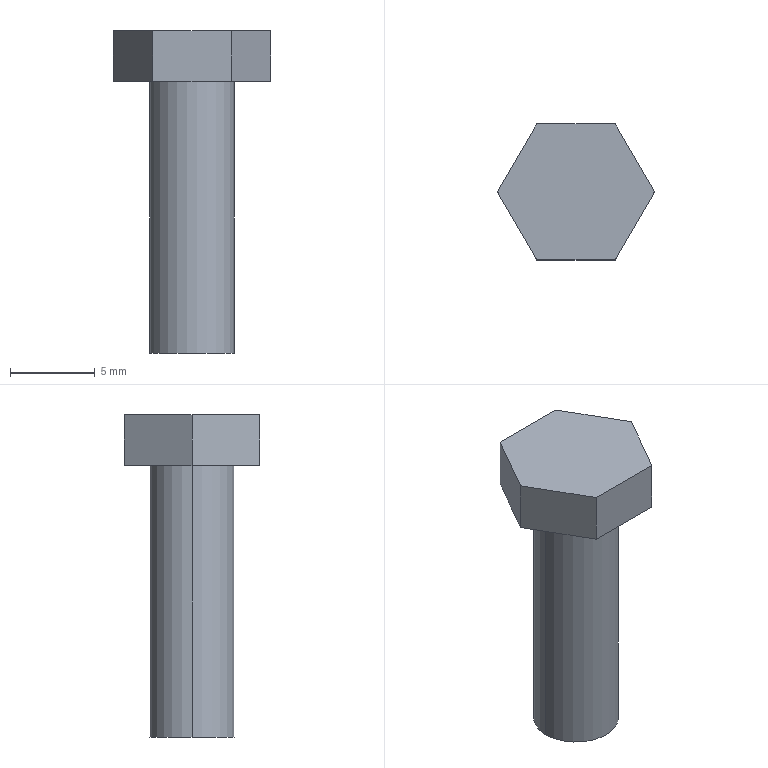Part | NX | features BREP 1 | 1 solid | 11 faces | box 9.238 x 8 x 19 mm | volume 480.436 mm3 | plane 9 | cylinder 2 | commonest cylinder face diameters 5 x2
STEP:
#1=CARTESIAN_POINT('',(2.5,-24.5,16.));
#2=VERTEX_POINT('',#1);
#3=CARTESIAN_POINT('',(-2.5,-24.5,16.));
#4=VERTEX_POINT('',#3);
#5=CARTESIAN_POINT('',(0.,-24.5,16.));
#6=DIRECTION('',(0.,0.,1.));
#7=DIRECTION('',(1.,0.,0.));
#8=AXIS2_PLACEMENT_3D('',#5,#6,#7);
#9=CIRCLE('',#8,2.5);
#10=EDGE_CURVE('',#2,#4,#9,.T.);
#11=ORIENTED_EDGE('',*,*,#10,.F.);
#12=CARTESIAN_POINT('',(2.5,-24.5,0.));
#13=VERTEX_POINT('',#12);
#14=CARTESIAN_POINT('',(2.5,-24.5,16.));
#15=DIRECTION('',(0.,0.,-1.));
#16=VECTOR('',#15,1000.);
#17=LINE('',#14,#16);
#18=EDGE_CURVE('',#2,#13,#17,.T.);
#19=ORIENTED_EDGE('',*,*,#18,.T.);
#20=CARTESIAN_POINT('',(-2.5,-24.5,0.));
#21=VERTEX_POINT('',#20);
#22=CARTESIAN_POINT('',(0.,-24.5,0.));
#23=DIRECTION('',(0.,0.,1.));
#24=DIRECTION('',(1.,0.,0.));
#25=AXIS2_PLACEMENT_3D('',#22,#23,#24);
#26=CIRCLE('',#25,2.5);
#27=EDGE_CURVE('',#13,#21,#26,.T.);
#28=ORIENTED_EDGE('',*,*,#27,.T.);
#29=CARTESIAN_POINT('',(-2.5,-24.5,16.));
#30=DIRECTION('',(0.,0.,-1.));
#31=VECTOR('',#30,1000.);
#32=LINE('',#29,#31);
#33=EDGE_CURVE('',#4,#21,#32,.T.);
#34=ORIENTED_EDGE('',*,*,#33,.F.);
#35=EDGE_LOOP('',(#11,#19,#28,#34));
#36=FACE_BOUND('',#35,.T.);
#37=CARTESIAN_POINT('',(0.,-24.5,16.));
#38=DIRECTION('',(0.,0.,-1.));
#39=DIRECTION('',(-1.,0.,0.));
#40=AXIS2_PLACEMENT_3D('',#37,#38,#39);
#41=CYLINDRICAL_SURFACE('',#40,2.5);
#42=ADVANCED_FACE('',(#36),#41,.T.);
#43=ORIENTED_EDGE('',*,*,#18,.F.);
#44=CARTESIAN_POINT('',(0.,-24.5,16.));
#45=DIRECTION('',(0.,0.,1.));
#46=DIRECTION('',(1.,0.,0.));
#47=AXIS2_PLACEMENT_3D('',#44,#45,#46);
#48=CIRCLE('',#47,2.5);
#49=EDGE_CURVE('',#4,#2,#48,.T.);
#50=ORIENTED_EDGE('',*,*,#49,.F.);
#51=ORIENTED_EDGE('',*,*,#33,.T.);
#52=CARTESIAN_POINT('',(0.,-24.5,0.));
#53=DIRECTION('',(0.,0.,1.));
#54=DIRECTION('',(1.,0.,0.));
#55=AXIS2_PLACEMENT_3D('',#52,#53,#54);
#56=CIRCLE('',#55,2.5);
#57=EDGE_CURVE('',#21,#13,#56,.T.);
#58=ORIENTED_EDGE('',*,*,#57,.T.);
#59=EDGE_LOOP('',(#43,#50,#51,#58));
#60=FACE_BOUND('',#59,.T.);
#61=CARTESIAN_POINT('',(0.,-24.5,16.));
#62=DIRECTION('',(0.,0.,-1.));
#63=DIRECTION('',(-1.,0.,0.));
#64=AXIS2_PLACEMENT_3D('',#61,#62,#63);
#65=CYLINDRICAL_SURFACE('',#64,2.5);
#66=ADVANCED_FACE('',(#60),#65,.T.);
#67=ORIENTED_EDGE('',*,*,#57,.F.);
#68=ORIENTED_EDGE('',*,*,#27,.F.);
#69=EDGE_LOOP('',(#67,#68));
#70=FACE_BOUND('',#69,.T.);
#71=CARTESIAN_POINT('',(0.,-24.5,0.));
#72=DIRECTION('',(0.,0.,1.));
#73=DIRECTION('',(1.,0.,0.));
#74=AXIS2_PLACEMENT_3D('',#71,#72,#73);
#75=PLANE('',#74);
#76=ADVANCED_FACE('',(#70),#75,.F.);
#77=CARTESIAN_POINT('',(4.619,-24.5,16.));
#78=VERTEX_POINT('',#77);
#79=CARTESIAN_POINT('',(2.309,-20.5,16.));
#80=VERTEX_POINT('',#79);
#81=CARTESIAN_POINT('',(4.619,-24.5,16.));
#82=DIRECTION('',(-0.5,0.866,0.));
#83=VECTOR('',#82,1000.);
#84=LINE('',#81,#83);
#85=EDGE_CURVE('',#78,#80,#84,.T.);
#86=ORIENTED_EDGE('',*,*,#85,.F.);
#87=CARTESIAN_POINT('',(2.309,-28.5,16.));
#88=VERTEX_POINT('',#87);
#89=CARTESIAN_POINT('',(2.309,-28.5,16.));
#90=DIRECTION('',(0.5,0.866,0.));
#91=VECTOR('',#90,1000.);
#92=LINE('',#89,#91);
#93=EDGE_CURVE('',#88,#78,#92,.T.);
#94=ORIENTED_EDGE('',*,*,#93,.F.);
#95=CARTESIAN_POINT('',(-2.309,-28.5,16.));
#96=VERTEX_POINT('',#95);
#97=CARTESIAN_POINT('',(-2.309,-28.5,16.));
#98=DIRECTION('',(1.,0.,0.));
#99=VECTOR('',#98,1000.);
#100=LINE('',#97,#99);
#101=EDGE_CURVE('',#96,#88,#100,.T.);
#102=ORIENTED_EDGE('',*,*,#101,.F.);
#103=CARTESIAN_POINT('',(-4.619,-24.5,16.));
#104=VERTEX_POINT('',#103);
#105=CARTESIAN_POINT('',(-4.619,-24.5,16.));
#106=DIRECTION('',(0.5,-0.866,0.));
#107=VECTOR('',#106,1000.);
#108=LINE('',#105,#107);
#109=EDGE_CURVE('',#104,#96,#108,.T.);
#110=ORIENTED_EDGE('',*,*,#109,.F.);
#111=CARTESIAN_POINT('',(-2.309,-20.5,16.));
#112=VERTEX_POINT('',#111);
#113=CARTESIAN_POINT('',(-2.309,-20.5,16.));
#114=DIRECTION('',(-0.5,-0.866,0.));
#115=VECTOR('',#114,1000.);
#116=LINE('',#113,#115);
#117=EDGE_CURVE('',#112,#104,#116,.T.);
#118=ORIENTED_EDGE('',*,*,#117,.F.);
#119=CARTESIAN_POINT('',(2.309,-20.5,16.));
#120=DIRECTION('',(-1.,0.,0.));
#121=VECTOR('',#120,1000.);
#122=LINE('',#119,#121);
#123=EDGE_CURVE('',#80,#112,#122,.T.);
#124=ORIENTED_EDGE('',*,*,#123,.F.);
#125=EDGE_LOOP('',(#86,#94,#102,#110,#118,#124));
#126=FACE_BOUND('',#125,.T.);
#127=ORIENTED_EDGE('',*,*,#49,.T.);
#128=ORIENTED_EDGE('',*,*,#10,.T.);
#129=EDGE_LOOP('',(#127,#128));
#130=FACE_BOUND('',#129,.T.);
#131=CARTESIAN_POINT('',(2.309,-20.5,16.));
#132=DIRECTION('',(0.,0.,1.));
#133=DIRECTION('',(1.,0.,0.));
#134=AXIS2_PLACEMENT_3D('',#131,#132,#133);
#135=PLANE('',#134);
#136=ADVANCED_FACE('',(#126,#130),#135,.F.);
#137=ORIENTED_EDGE('',*,*,#85,.T.);
#138=CARTESIAN_POINT('',(2.309,-20.5,19.));
#139=VERTEX_POINT('',#138);
#140=CARTESIAN_POINT('',(2.309,-20.5,19.));
#141=DIRECTION('',(0.,0.,-1.));
#142=VECTOR('',#141,1000.);
#143=LINE('',#140,#142);
#144=EDGE_CURVE('',#139,#80,#143,.T.);
#145=ORIENTED_EDGE('',*,*,#144,.F.);
#146=CARTESIAN_POINT('',(4.619,-24.5,19.));
#147=VERTEX_POINT('',#146);
#148=CARTESIAN_POINT('',(4.619,-24.5,19.));
#149=DIRECTION('',(-0.5,0.866,0.));
#150=VECTOR('',#149,1000.);
#151=LINE('',#148,#150);
#152=EDGE_CURVE('',#147,#139,#151,.T.);
#153=ORIENTED_EDGE('',*,*,#152,.F.);
#154=CARTESIAN_POINT('',(4.619,-24.5,19.));
#155=DIRECTION('',(0.,0.,-1.));
#156=VECTOR('',#155,1000.);
#157=LINE('',#154,#156);
#158=EDGE_CURVE('',#147,#78,#157,.T.);
#159=ORIENTED_EDGE('',*,*,#158,.T.);
#160=EDGE_LOOP('',(#137,#145,#153,#159));
#161=FACE_BOUND('',#160,.T.);
#162=CARTESIAN_POINT('',(4.619,-24.5,19.));
#163=DIRECTION('',(-0.866,-0.5,0.));
#164=DIRECTION('',(-0.5,0.866,0.));
#165=AXIS2_PLACEMENT_3D('',#162,#163,#164);
#166=PLANE('',#165);
#167=ADVANCED_FACE('',(#161),#166,.F.);
#168=ORIENTED_EDGE('',*,*,#123,.T.);
#169=CARTESIAN_POINT('',(-2.309,-20.5,19.));
#170=VERTEX_POINT('',#169);
#171=CARTESIAN_POINT('',(-2.309,-20.5,19.));
#172=DIRECTION('',(0.,0.,-1.));
#173=VECTOR('',#172,1000.);
#174=LINE('',#171,#173);
#175=EDGE_CURVE('',#170,#112,#174,.T.);
#176=ORIENTED_EDGE('',*,*,#175,.F.);
#177=CARTESIAN_POINT('',(2.309,-20.5,19.));
#178=DIRECTION('',(-1.,0.,0.));
#179=VECTOR('',#178,1000.);
#180=LINE('',#177,#179);
#181=EDGE_CURVE('',#139,#170,#180,.T.);
#182=ORIENTED_EDGE('',*,*,#181,.F.);
#183=ORIENTED_EDGE('',*,*,#144,.T.);
#184=EDGE_LOOP('',(#168,#176,#182,#183));
#185=FACE_BOUND('',#184,.T.);
#186=CARTESIAN_POINT('',(2.309,-20.5,19.));
#187=DIRECTION('',(0.,-1.,0.));
#188=DIRECTION('',(0.,0.,-1.));
#189=AXIS2_PLACEMENT_3D('',#186,#187,#188);
#190=PLANE('',#189);
#191=ADVANCED_FACE('',(#185),#190,.F.);
#192=ORIENTED_EDGE('',*,*,#117,.T.);
#193=CARTESIAN_POINT('',(-4.619,-24.5,19.));
#194=VERTEX_POINT('',#193);
#195=CARTESIAN_POINT('',(-4.619,-24.5,19.));
#196=DIRECTION('',(0.,0.,-1.));
#197=VECTOR('',#196,1000.);
#198=LINE('',#195,#197);
#199=EDGE_CURVE('',#194,#104,#198,.T.);
#200=ORIENTED_EDGE('',*,*,#199,.F.);
#201=CARTESIAN_POINT('',(-2.309,-20.5,19.));
#202=DIRECTION('',(-0.5,-0.866,0.));
#203=VECTOR('',#202,1000.);
#204=LINE('',#201,#203);
#205=EDGE_CURVE('',#170,#194,#204,.T.);
#206=ORIENTED_EDGE('',*,*,#205,.F.);
#207=ORIENTED_EDGE('',*,*,#175,.T.);
#208=EDGE_LOOP('',(#192,#200,#206,#207));
#209=FACE_BOUND('',#208,.T.);
#210=CARTESIAN_POINT('',(-2.309,-20.5,19.));
#211=DIRECTION('',(0.866,-0.5,0.));
#212=DIRECTION('',(0.,0.,-1.));
#213=AXIS2_PLACEMENT_3D('',#210,#211,#212);
#214=PLANE('',#213);
#215=ADVANCED_FACE('',(#209),#214,.F.);
#216=ORIENTED_EDGE('',*,*,#109,.T.);
#217=CARTESIAN_POINT('',(-2.309,-28.5,19.));
#218=VERTEX_POINT('',#217);
#219=CARTESIAN_POINT('',(-2.309,-28.5,19.));
#220=DIRECTION('',(0.,0.,-1.));
#221=VECTOR('',#220,1000.);
#222=LINE('',#219,#221);
#223=EDGE_CURVE('',#218,#96,#222,.T.);
#224=ORIENTED_EDGE('',*,*,#223,.F.);
#225=CARTESIAN_POINT('',(-4.619,-24.5,19.));
#226=DIRECTION('',(0.5,-0.866,0.));
#227=VECTOR('',#226,1000.);
#228=LINE('',#225,#227);
#229=EDGE_CURVE('',#194,#218,#228,.T.);
#230=ORIENTED_EDGE('',*,*,#229,.F.);
#231=ORIENTED_EDGE('',*,*,#199,.T.);
#232=EDGE_LOOP('',(#216,#224,#230,#231));
#233=FACE_BOUND('',#232,.T.);
#234=CARTESIAN_POINT('',(-4.619,-24.5,19.));
#235=DIRECTION('',(0.866,0.5,0.));
#236=DIRECTION('',(0.,0.,-1.));
#237=AXIS2_PLACEMENT_3D('',#234,#235,#236);
#238=PLANE('',#237);
#239=ADVANCED_FACE('',(#233),#238,.F.);
#240=ORIENTED_EDGE('',*,*,#101,.T.);
#241=CARTESIAN_POINT('',(2.309,-28.5,19.));
#242=VERTEX_POINT('',#241);
#243=CARTESIAN_POINT('',(2.309,-28.5,19.));
#244=DIRECTION('',(0.,0.,-1.));
#245=VECTOR('',#244,1000.);
#246=LINE('',#243,#245);
#247=EDGE_CURVE('',#242,#88,#246,.T.);
#248=ORIENTED_EDGE('',*,*,#247,.F.);
#249=CARTESIAN_POINT('',(-2.309,-28.5,19.));
#250=DIRECTION('',(1.,0.,0.));
#251=VECTOR('',#250,1000.);
#252=LINE('',#249,#251);
#253=EDGE_CURVE('',#218,#242,#252,.T.);
#254=ORIENTED_EDGE('',*,*,#253,.F.);
#255=ORIENTED_EDGE('',*,*,#223,.T.);
#256=EDGE_LOOP('',(#240,#248,#254,#255));
#257=FACE_BOUND('',#256,.T.);
#258=CARTESIAN_POINT('',(-2.309,-28.5,19.));
#259=DIRECTION('',(0.,1.,0.));
#260=DIRECTION('',(1.,0.,0.));
#261=AXIS2_PLACEMENT_3D('',#258,#259,#260);
#262=PLANE('',#261);
#263=ADVANCED_FACE('',(#257),#262,.F.);
#264=ORIENTED_EDGE('',*,*,#93,.T.);
#265=ORIENTED_EDGE('',*,*,#158,.F.);
#266=CARTESIAN_POINT('',(2.309,-28.5,19.));
#267=DIRECTION('',(0.5,0.866,0.));
#268=VECTOR('',#267,1000.);
#269=LINE('',#266,#268);
#270=EDGE_CURVE('',#242,#147,#269,.T.);
#271=ORIENTED_EDGE('',*,*,#270,.F.);
#272=ORIENTED_EDGE('',*,*,#247,.T.);
#273=EDGE_LOOP('',(#264,#265,#271,#272));
#274=FACE_BOUND('',#273,.T.);
#275=CARTESIAN_POINT('',(2.309,-28.5,19.));
#276=DIRECTION('',(-0.866,0.5,0.));
#277=DIRECTION('',(0.,0.,1.));
#278=AXIS2_PLACEMENT_3D('',#275,#276,#277);
#279=PLANE('',#278);
#280=ADVANCED_FACE('',(#274),#279,.F.);
#281=ORIENTED_EDGE('',*,*,#152,.T.);
#282=ORIENTED_EDGE('',*,*,#181,.T.);
#283=ORIENTED_EDGE('',*,*,#205,.T.);
#284=ORIENTED_EDGE('',*,*,#229,.T.);
#285=ORIENTED_EDGE('',*,*,#253,.T.);
#286=ORIENTED_EDGE('',*,*,#270,.T.);
#287=EDGE_LOOP('',(#281,#282,#283,#284,#285,#286));
#288=FACE_BOUND('',#287,.T.);
#289=CARTESIAN_POINT('',(2.309,-20.5,19.));
#290=DIRECTION('',(0.,0.,1.));
#291=DIRECTION('',(1.,0.,0.));
#292=AXIS2_PLACEMENT_3D('',#289,#290,#291);
#293=PLANE('',#292);
#294=ADVANCED_FACE('',(#288),#293,.T.);
#295=CLOSED_SHELL('',(#42,#66,#76,#136,#167,#191,#215,#239,#263,#280,#294));
#296=MANIFOLD_SOLID_BREP('',#295);
#297=(LENGTH_UNIT()NAMED_UNIT(*)SI_UNIT(.MILLI.,.METRE.));
#298=UNCERTAINTY_MEASURE_WITH_UNIT(LENGTH_MEASURE(0.00001),#297,'','');
#299=(NAMED_UNIT(*)PLANE_ANGLE_UNIT()SI_UNIT($,.RADIAN.));
#300=(NAMED_UNIT(*)SI_UNIT($,.STERADIAN.)SOLID_ANGLE_UNIT());
#301=(GEOMETRIC_REPRESENTATION_CONTEXT(3)GLOBAL_UNCERTAINTY_ASSIGNED_CONTEXT((#298))GLOBAL_UNIT_ASSIGNED_CONTEXT((#297,#299,#300))REPRESENTATION_CONTEXT('',''));
#302=ADVANCED_BREP_SHAPE_REPRESENTATION('',(#296),#301);